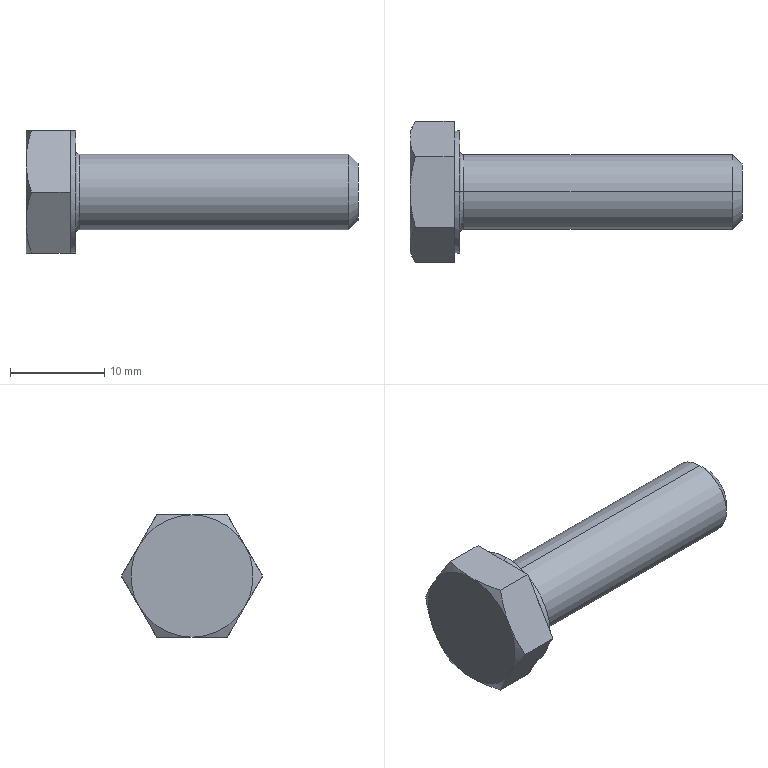Part | SolidWorks | features RevCut 4, Chamfer 1, Extrusion 1, Fillet 1, LPattern 1, Revolution 1 | 1 solid | 29 faces | box 35.3 x 15.011 x 13 mm | volume 2262 mm3 | plane 15 | cone 8 | cylinder 4 | torus 2 | commonest cylinder face diameters 8 x2 13 x2
STEP:
#1=CARTESIAN_POINT('',(5.7,0.,4.));
#2=VERTEX_POINT('',#1);
#3=CARTESIAN_POINT('',(5.7,0.,-4.));
#4=VERTEX_POINT('',#3);
#5=CARTESIAN_POINT('',(5.7,0.,0.));
#6=DIRECTION('',(1.,0.,0.));
#7=DIRECTION('',(0.,0.,-1.));
#8=AXIS2_PLACEMENT_3D('',#5,#6,#7);
#9=CIRCLE('',#8,4.);
#10=EDGE_CURVE('',#2,#4,#9,.T.);
#11=ORIENTED_EDGE('',*,*,#10,.F.);
#12=CARTESIAN_POINT('',(5.3,0.,4.4));
#13=VERTEX_POINT('',#12);
#14=CARTESIAN_POINT('',(5.7,0.,4.4));
#15=DIRECTION('',(0.,1.,0.));
#16=DIRECTION('',(0.,0.,1.));
#17=AXIS2_PLACEMENT_3D('',#14,#15,#16);
#18=CIRCLE('',#17,0.4);
#19=EDGE_CURVE('',#2,#13,#18,.T.);
#20=ORIENTED_EDGE('',*,*,#19,.T.);
#21=CARTESIAN_POINT('',(5.3,0.,-4.4));
#22=VERTEX_POINT('',#21);
#23=CARTESIAN_POINT('',(5.3,0.,0.));
#24=DIRECTION('',(-1.,0.,0.));
#25=DIRECTION('',(0.,0.,-1.));
#26=AXIS2_PLACEMENT_3D('',#23,#24,#25);
#27=CIRCLE('',#26,4.4);
#28=EDGE_CURVE('',#22,#13,#27,.T.);
#29=ORIENTED_EDGE('',*,*,#28,.F.);
#30=CARTESIAN_POINT('',(5.7,0.,-4.4));
#31=DIRECTION('',(0.,-1.,0.));
#32=DIRECTION('',(0.,0.,-1.));
#33=AXIS2_PLACEMENT_3D('',#30,#31,#32);
#34=CIRCLE('',#33,0.4);
#35=EDGE_CURVE('',#4,#22,#34,.T.);
#36=ORIENTED_EDGE('',*,*,#35,.F.);
#37=EDGE_LOOP('',(#11,#20,#29,#36));
#38=FACE_OUTER_BOUND('',#37,.T.);
#39=CARTESIAN_POINT('',(5.7,0.,0.));
#40=DIRECTION('',(1.,0.,0.));
#41=DIRECTION('',(0.,0.,-1.));
#42=AXIS2_PLACEMENT_3D('',#39,#40,#41);
#43=TOROIDAL_SURFACE('',#42,4.4,0.4);
#44=ADVANCED_FACE('',(#38),#43,.F.);
#45=CARTESIAN_POINT('',(35.3,0.,-3.));
#46=VERTEX_POINT('',#45);
#47=CARTESIAN_POINT('',(35.3,0.,3.));
#48=VERTEX_POINT('',#47);
#49=CARTESIAN_POINT('',(35.3,0.,0.));
#50=DIRECTION('',(1.,0.,0.));
#51=DIRECTION('',(0.,0.,1.));
#52=AXIS2_PLACEMENT_3D('',#49,#50,#51);
#53=CIRCLE('',#52,3.);
#54=EDGE_CURVE('',#46,#48,#53,.T.);
#55=ORIENTED_EDGE('',*,*,#54,.F.);
#56=CARTESIAN_POINT('',(34.3,0.,-4.));
#57=VERTEX_POINT('',#56);
#58=CARTESIAN_POINT('',(34.3,0.,-4.));
#59=DIRECTION('',(-0.7071,0.,-0.7071));
#60=VECTOR('',#59,1000.);
#61=LINE('',#58,#60);
#62=EDGE_CURVE('',#46,#57,#61,.T.);
#63=ORIENTED_EDGE('',*,*,#62,.T.);
#64=CARTESIAN_POINT('',(34.3,0.,4.));
#65=VERTEX_POINT('',#64);
#66=CARTESIAN_POINT('',(34.3,0.,0.));
#67=DIRECTION('',(-1.,0.,0.));
#68=DIRECTION('',(0.,0.,1.));
#69=AXIS2_PLACEMENT_3D('',#66,#67,#68);
#70=CIRCLE('',#69,4.);
#71=EDGE_CURVE('',#65,#57,#70,.T.);
#72=ORIENTED_EDGE('',*,*,#71,.F.);
#73=CARTESIAN_POINT('',(34.3,0.,4.));
#74=DIRECTION('',(-0.7071,0.,0.7071));
#75=VECTOR('',#74,1000.);
#76=LINE('',#73,#75);
#77=EDGE_CURVE('',#48,#65,#76,.T.);
#78=ORIENTED_EDGE('',*,*,#77,.F.);
#79=EDGE_LOOP('',(#55,#63,#72,#78));
#80=FACE_OUTER_BOUND('',#79,.T.);
#81=CARTESIAN_POINT('',(34.3,0.,0.));
#82=DIRECTION('',(-1.,0.,0.));
#83=DIRECTION('',(0.,0.,1.));
#84=AXIS2_PLACEMENT_3D('',#81,#82,#83);
#85=CONICAL_SURFACE('',#84,4.,0.7854);
#86=ADVANCED_FACE('',(#80),#85,.T.);
#87=ORIENTED_EDGE('',*,*,#71,.T.);
#88=CARTESIAN_POINT('',(0.,0.,-4.));
#89=DIRECTION('',(-1.,0.,0.));
#90=VECTOR('',#89,1000.);
#91=LINE('',#88,#90);
#92=EDGE_CURVE('',#57,#4,#91,.T.);
#93=ORIENTED_EDGE('',*,*,#92,.T.);
#94=CARTESIAN_POINT('',(5.7,0.,0.));
#95=DIRECTION('',(1.,0.,0.));
#96=DIRECTION('',(0.,0.,-1.));
#97=AXIS2_PLACEMENT_3D('',#94,#95,#96);
#98=CIRCLE('',#97,4.);
#99=EDGE_CURVE('',#4,#2,#98,.T.);
#100=ORIENTED_EDGE('',*,*,#99,.T.);
#101=CARTESIAN_POINT('',(0.,0.,4.));
#102=DIRECTION('',(-1.,0.,0.));
#103=VECTOR('',#102,1000.);
#104=LINE('',#101,#103);
#105=EDGE_CURVE('',#65,#2,#104,.T.);
#106=ORIENTED_EDGE('',*,*,#105,.F.);
#107=EDGE_LOOP('',(#87,#93,#100,#106));
#108=FACE_OUTER_BOUND('',#107,.T.);
#109=CARTESIAN_POINT('',(0.,0.,0.));
#110=DIRECTION('',(-1.,0.,0.));
#111=DIRECTION('',(0.,0.,1.));
#112=AXIS2_PLACEMENT_3D('',#109,#110,#111);
#113=CYLINDRICAL_SURFACE('',#112,4.);
#114=ADVANCED_FACE('',(#108),#113,.T.);
#115=CARTESIAN_POINT('',(5.3,0.,-6.5));
#116=VERTEX_POINT('',#115);
#117=CARTESIAN_POINT('',(5.3,0.,6.5));
#118=VERTEX_POINT('',#117);
#119=CARTESIAN_POINT('',(5.3,0.,0.));
#120=DIRECTION('',(1.,0.,0.));
#121=DIRECTION('',(0.,0.,-1.));
#122=AXIS2_PLACEMENT_3D('',#119,#120,#121);
#123=CIRCLE('',#122,6.5);
#124=EDGE_CURVE('',#116,#118,#123,.T.);
#125=ORIENTED_EDGE('',*,*,#124,.F.);
#126=CARTESIAN_POINT('',(4.7,0.,-6.5));
#127=VERTEX_POINT('',#126);
#128=CARTESIAN_POINT('',(0.,0.,-6.5));
#129=DIRECTION('',(-1.,0.,0.));
#130=VECTOR('',#129,1000.);
#131=LINE('',#128,#130);
#132=EDGE_CURVE('',#116,#127,#131,.T.);
#133=ORIENTED_EDGE('',*,*,#132,.T.);
#134=CARTESIAN_POINT('',(4.7,5.629,-3.25));
#135=VERTEX_POINT('',#134);
#136=CARTESIAN_POINT('',(4.7,0.,0.));
#137=DIRECTION('',(-1.,0.,0.));
#138=DIRECTION('',(0.,0.,1.));
#139=AXIS2_PLACEMENT_3D('',#136,#137,#138);
#140=CIRCLE('',#139,6.5);
#141=EDGE_CURVE('',#135,#127,#140,.T.);
#142=ORIENTED_EDGE('',*,*,#141,.F.);
#143=CARTESIAN_POINT('',(4.7,5.629,3.25));
#144=VERTEX_POINT('',#143);
#145=CARTESIAN_POINT('',(4.7,0.,0.));
#146=DIRECTION('',(-1.,0.,0.));
#147=DIRECTION('',(0.,0.,1.));
#148=AXIS2_PLACEMENT_3D('',#145,#146,#147);
#149=CIRCLE('',#148,6.5);
#150=EDGE_CURVE('',#144,#135,#149,.T.);
#151=ORIENTED_EDGE('',*,*,#150,.F.);
#152=CARTESIAN_POINT('',(4.7,0.,6.5));
#153=VERTEX_POINT('',#152);
#154=CARTESIAN_POINT('',(4.7,0.,0.));
#155=DIRECTION('',(-1.,0.,0.));
#156=DIRECTION('',(0.,0.,1.));
#157=AXIS2_PLACEMENT_3D('',#154,#155,#156);
#158=CIRCLE('',#157,6.5);
#159=EDGE_CURVE('',#153,#144,#158,.T.);
#160=ORIENTED_EDGE('',*,*,#159,.F.);
#161=CARTESIAN_POINT('',(0.,0.,6.5));
#162=DIRECTION('',(-1.,0.,0.));
#163=VECTOR('',#162,1000.);
#164=LINE('',#161,#163);
#165=EDGE_CURVE('',#118,#153,#164,.T.);
#166=ORIENTED_EDGE('',*,*,#165,.F.);
#167=EDGE_LOOP('',(#125,#133,#142,#151,#160,#166));
#168=FACE_OUTER_BOUND('',#167,.T.);
#169=CARTESIAN_POINT('',(0.,0.,0.));
#170=DIRECTION('',(-1.,0.,0.));
#171=DIRECTION('',(0.,0.,1.));
#172=AXIS2_PLACEMENT_3D('',#169,#170,#171);
#173=CYLINDRICAL_SURFACE('',#172,6.5);
#174=ADVANCED_FACE('',(#168),#173,.T.);
#175=CARTESIAN_POINT('',(4.7,3.753,-6.5));
#176=VERTEX_POINT('',#175);
#177=CARTESIAN_POINT('',(4.7,3.753,-6.5));
#178=DIRECTION('',(0.,0.5,0.866));
#179=VECTOR('',#178,1000.);
#180=LINE('',#177,#179);
#181=EDGE_CURVE('',#176,#135,#180,.T.);
#182=ORIENTED_EDGE('',*,*,#181,.F.);
#183=CARTESIAN_POINT('',(0.5806,3.753,-6.5));
#184=VERTEX_POINT('',#183);
#185=CARTESIAN_POINT('',(5.3,3.753,-6.5));
#186=DIRECTION('',(-1.,0.,0.));
#187=VECTOR('',#186,1000.);
#188=LINE('',#185,#187);
#189=EDGE_CURVE('',#176,#184,#188,.T.);
#190=ORIENTED_EDGE('',*,*,#189,.T.);
#191=CARTESIAN_POINT('',(0.,5.629,-3.25));
#192=VERTEX_POINT('',#191);
#193=CARTESIAN_POINT('',(0.,5.629,-3.25));
#194=CARTESIAN_POINT('',(0.,5.47,-3.526));
#195=CARTESIAN_POINT('',(0.01372,5.31,-3.803));
#196=CARTESIAN_POINT('',(0.06683,4.994,-4.351));
#197=CARTESIAN_POINT('',(0.1062,4.836,-4.623));
#198=CARTESIAN_POINT('',(0.2578,4.368,-5.435));
#199=CARTESIAN_POINT('',(0.4038,4.059,-5.97));
#200=CARTESIAN_POINT('',(0.5806,3.753,-6.5));
#201=B_SPLINE_CURVE_WITH_KNOTS('',3,(#193,#194,#195,#196,#197,#198,#199,#200),.UNSPECIFIED.,.F.,.F.,(4,2,2,4),(0.003797,0.004743,0.005689,0.00758),.UNSPECIFIED.);
#202=EDGE_CURVE('',#192,#184,#201,.T.);
#203=ORIENTED_EDGE('',*,*,#202,.F.);
#204=CARTESIAN_POINT('',(0.5806,7.506,0.));
#205=VERTEX_POINT('',#204);
#206=CARTESIAN_POINT('',(0.5806,7.506,0.));
#207=CARTESIAN_POINT('',(0.4033,7.199,-0.5317));
#208=CARTESIAN_POINT('',(0.2573,6.889,-1.067));
#209=CARTESIAN_POINT('',(0.05533,6.265,-2.149));
#210=CARTESIAN_POINT('',(0.,5.949,-2.696));
#211=CARTESIAN_POINT('',(0.,5.629,-3.25));
#212=B_SPLINE_CURVE_WITH_KNOTS('',3,(#206,#207,#208,#209,#210,#211),.UNSPECIFIED.,.F.,.F.,(4,2,4),(0.000000238,0.001899,0.003797),.UNSPECIFIED.);
#213=EDGE_CURVE('',#205,#192,#212,.T.);
#214=ORIENTED_EDGE('',*,*,#213,.F.);
#215=CARTESIAN_POINT('',(4.7,7.506,0.));
#216=VERTEX_POINT('',#215);
#217=CARTESIAN_POINT('',(5.3,7.506,0.));
#218=DIRECTION('',(-1.,0.,0.));
#219=VECTOR('',#218,1000.);
#220=LINE('',#217,#219);
#221=EDGE_CURVE('',#216,#205,#220,.T.);
#222=ORIENTED_EDGE('',*,*,#221,.F.);
#223=CARTESIAN_POINT('',(4.7,3.753,-6.5));
#224=DIRECTION('',(0.,0.5,0.866));
#225=VECTOR('',#224,1000.);
#226=LINE('',#223,#225);
#227=EDGE_CURVE('',#135,#216,#226,.T.);
#228=ORIENTED_EDGE('',*,*,#227,.F.);
#229=EDGE_LOOP('',(#182,#190,#203,#214,#222,#228));
#230=FACE_OUTER_BOUND('',#229,.T.);
#231=CARTESIAN_POINT('',(5.3,3.753,-6.5));
#232=DIRECTION('',(0.,-0.866,0.5));
#233=DIRECTION('',(0.,-0.5,-0.866));
#234=AXIS2_PLACEMENT_3D('',#231,#232,#233);
#235=PLANE('',#234);
#236=ADVANCED_FACE('',(#230),#235,.F.);
#237=CARTESIAN_POINT('',(4.7,7.506,0.));
#238=DIRECTION('',(0.,-0.5,0.866));
#239=VECTOR('',#238,1000.);
#240=LINE('',#237,#239);
#241=EDGE_CURVE('',#216,#144,#240,.T.);
#242=ORIENTED_EDGE('',*,*,#241,.F.);
#243=ORIENTED_EDGE('',*,*,#221,.T.);
#244=CARTESIAN_POINT('',(0.,5.629,3.25));
#245=VERTEX_POINT('',#244);
#246=CARTESIAN_POINT('',(0.,5.629,3.25));
#247=CARTESIAN_POINT('',(0.,5.788,2.974));
#248=CARTESIAN_POINT('',(0.01372,5.948,2.697));
#249=CARTESIAN_POINT('',(0.06683,6.265,2.149));
#250=CARTESIAN_POINT('',(0.1062,6.422,1.877));
#251=CARTESIAN_POINT('',(0.2578,6.891,1.065));
#252=CARTESIAN_POINT('',(0.4038,7.199,0.5303));
#253=CARTESIAN_POINT('',(0.5806,7.506,0.));
#254=B_SPLINE_CURVE_WITH_KNOTS('',3,(#246,#247,#248,#249,#250,#251,#252,#253),.UNSPECIFIED.,.F.,.F.,(4,2,2,4),(0.003797,0.004743,0.005689,0.00758),.UNSPECIFIED.);
#255=EDGE_CURVE('',#245,#205,#254,.T.);
#256=ORIENTED_EDGE('',*,*,#255,.F.);
#257=CARTESIAN_POINT('',(0.5806,3.753,6.5));
#258=VERTEX_POINT('',#257);
#259=CARTESIAN_POINT('',(0.5806,3.753,6.5));
#260=CARTESIAN_POINT('',(0.4033,4.06,5.968));
#261=CARTESIAN_POINT('',(0.2573,4.369,5.433));
#262=CARTESIAN_POINT('',(0.05533,4.994,4.351));
#263=CARTESIAN_POINT('',(0.,5.309,3.804));
#264=CARTESIAN_POINT('',(0.,5.629,3.25));
#265=B_SPLINE_CURVE_WITH_KNOTS('',3,(#259,#260,#261,#262,#263,#264),.UNSPECIFIED.,.F.,.F.,(4,2,4),(0.000000238,0.001899,0.003797),.UNSPECIFIED.);
#266=EDGE_CURVE('',#258,#245,#265,.T.);
#267=ORIENTED_EDGE('',*,*,#266,.F.);
#268=CARTESIAN_POINT('',(4.7,3.753,6.5));
#269=VERTEX_POINT('',#268);
#270=CARTESIAN_POINT('',(5.3,3.753,6.5));
#271=DIRECTION('',(-1.,0.,0.));
#272=VECTOR('',#271,1000.);
#273=LINE('',#270,#272);
#274=EDGE_CURVE('',#269,#258,#273,.T.);
#275=ORIENTED_EDGE('',*,*,#274,.F.);
#276=CARTESIAN_POINT('',(4.7,7.506,0.));
#277=DIRECTION('',(0.,-0.5,0.866));
#278=VECTOR('',#277,1000.);
#279=LINE('',#276,#278);
#280=EDGE_CURVE('',#144,#269,#279,.T.);
#281=ORIENTED_EDGE('',*,*,#280,.F.);
#282=EDGE_LOOP('',(#242,#243,#256,#267,#275,#281));
#283=FACE_OUTER_BOUND('',#282,.T.);
#284=CARTESIAN_POINT('',(5.3,7.506,0.));
#285=DIRECTION('',(0.,-0.866,-0.5));
#286=DIRECTION('',(0.,0.5,-0.866));
#287=AXIS2_PLACEMENT_3D('',#284,#285,#286);
#288=PLANE('',#287);
#289=ADVANCED_FACE('',(#283),#288,.F.);
#290=CARTESIAN_POINT('',(4.7,3.753,6.5));
#291=DIRECTION('',(0.,-1.,0.));
#292=VECTOR('',#291,1000.);
#293=LINE('',#290,#292);
#294=EDGE_CURVE('',#269,#153,#293,.T.);
#295=ORIENTED_EDGE('',*,*,#294,.F.);
#296=ORIENTED_EDGE('',*,*,#274,.T.);
#297=CARTESIAN_POINT('',(0.,0.,6.5));
#298=VERTEX_POINT('',#297);
#299=CARTESIAN_POINT('',(0.,0.,6.5));
#300=CARTESIAN_POINT('',(0.,0.6351,6.5));
#301=CARTESIAN_POINT('',(0.05613,1.279,6.5));
#302=CARTESIAN_POINT('',(0.2595,2.531,6.5));
#303=CARTESIAN_POINT('',(0.4054,3.146,6.5));
#304=CARTESIAN_POINT('',(0.5806,3.753,6.5));
#305=B_SPLINE_CURVE_WITH_KNOTS('',3,(#299,#300,#301,#302,#303,#304),.UNSPECIFIED.,.F.,.F.,(4,2,4),(0.01067,0.01257,0.01447),.UNSPECIFIED.);
#306=EDGE_CURVE('',#298,#258,#305,.T.);
#307=ORIENTED_EDGE('',*,*,#306,.F.);
#308=CARTESIAN_POINT('',(0.5806,-3.753,6.5));
#309=VERTEX_POINT('',#308);
#310=CARTESIAN_POINT('',(0.5806,-3.753,6.5));
#311=CARTESIAN_POINT('',(0.4042,-3.142,6.5));
#312=CARTESIAN_POINT('',(0.2565,-2.517,6.5));
#313=CARTESIAN_POINT('',(0.05459,-1.265,6.5));
#314=CARTESIAN_POINT('',(0.,-0.6347,6.5));
#315=CARTESIAN_POINT('',(0.,0.,6.5));
#316=B_SPLINE_CURVE_WITH_KNOTS('',3,(#310,#311,#312,#313,#314,#315),.UNSPECIFIED.,.F.,.F.,(4,2,4),(0.006874,0.008773,0.01067),.UNSPECIFIED.);
#317=EDGE_CURVE('',#309,#298,#316,.T.);
#318=ORIENTED_EDGE('',*,*,#317,.F.);
#319=CARTESIAN_POINT('',(4.7,-3.753,6.5));
#320=VERTEX_POINT('',#319);
#321=CARTESIAN_POINT('',(5.3,-3.753,6.5));
#322=DIRECTION('',(-1.,0.,0.));
#323=VECTOR('',#322,1000.);
#324=LINE('',#321,#323);
#325=EDGE_CURVE('',#320,#309,#324,.T.);
#326=ORIENTED_EDGE('',*,*,#325,.F.);
#327=CARTESIAN_POINT('',(4.7,3.753,6.5));
#328=DIRECTION('',(0.,-1.,0.));
#329=VECTOR('',#328,1000.);
#330=LINE('',#327,#329);
#331=EDGE_CURVE('',#153,#320,#330,.T.);
#332=ORIENTED_EDGE('',*,*,#331,.F.);
#333=EDGE_LOOP('',(#295,#296,#307,#318,#326,#332));
#334=FACE_OUTER_BOUND('',#333,.T.);
#335=CARTESIAN_POINT('',(5.3,3.753,6.5));
#336=DIRECTION('',(0.,0.,-1.));
#337=DIRECTION('',(-1.,0.,0.));
#338=AXIS2_PLACEMENT_3D('',#335,#336,#337);
#339=PLANE('',#338);
#340=ADVANCED_FACE('',(#334),#339,.F.);
#341=CARTESIAN_POINT('',(4.7,-5.629,3.25));
#342=VERTEX_POINT('',#341);
#343=CARTESIAN_POINT('',(4.7,-7.506,0.));
#344=DIRECTION('',(0.,-0.5,-0.866));
#345=VECTOR('',#344,1000.);
#346=LINE('',#343,#345);
#347=EDGE_CURVE('',#320,#342,#346,.T.);
#348=ORIENTED_EDGE('',*,*,#347,.F.);
#349=ORIENTED_EDGE('',*,*,#325,.T.);
#350=CARTESIAN_POINT('',(0.,-5.629,3.25));
#351=VERTEX_POINT('',#350);
#352=CARTESIAN_POINT('',(0.,-5.629,3.25));
#353=CARTESIAN_POINT('',(0.,-5.47,3.526));
#354=CARTESIAN_POINT('',(0.01372,-5.31,3.803));
#355=CARTESIAN_POINT('',(0.06683,-4.994,4.351));
#356=CARTESIAN_POINT('',(0.1062,-4.836,4.623));
#357=CARTESIAN_POINT('',(0.2578,-4.368,5.435));
#358=CARTESIAN_POINT('',(0.4038,-4.059,5.97));
#359=CARTESIAN_POINT('',(0.5806,-3.753,6.5));
#360=B_SPLINE_CURVE_WITH_KNOTS('',3,(#352,#353,#354,#355,#356,#357,#358,#359),.UNSPECIFIED.,.F.,.F.,(4,2,2,4),(0.003797,0.004743,0.005689,0.00758),.UNSPECIFIED.);
#361=EDGE_CURVE('',#351,#309,#360,.T.);
#362=ORIENTED_EDGE('',*,*,#361,.F.);
#363=CARTESIAN_POINT('',(0.5806,-7.506,0.));
#364=VERTEX_POINT('',#363);
#365=CARTESIAN_POINT('',(0.5806,-7.506,0.));
#366=CARTESIAN_POINT('',(0.4033,-7.199,0.5317));
#367=CARTESIAN_POINT('',(0.2573,-6.889,1.067));
#368=CARTESIAN_POINT('',(0.05533,-6.265,2.149));
#369=CARTESIAN_POINT('',(0.,-5.949,2.696));
#370=CARTESIAN_POINT('',(0.,-5.629,3.25));
#371=B_SPLINE_CURVE_WITH_KNOTS('',3,(#365,#366,#367,#368,#369,#370),.UNSPECIFIED.,.F.,.F.,(4,2,4),(0.000000238,0.001899,0.003797),.UNSPECIFIED.);
#372=EDGE_CURVE('',#364,#351,#371,.T.);
#373=ORIENTED_EDGE('',*,*,#372,.F.);
#374=CARTESIAN_POINT('',(4.7,-7.506,0.));
#375=VERTEX_POINT('',#374);
#376=CARTESIAN_POINT('',(5.3,-7.506,0.));
#377=DIRECTION('',(-1.,0.,0.));
#378=VECTOR('',#377,1000.);
#379=LINE('',#376,#378);
#380=EDGE_CURVE('',#375,#364,#379,.T.);
#381=ORIENTED_EDGE('',*,*,#380,.F.);
#382=CARTESIAN_POINT('',(4.7,-7.506,0.));
#383=DIRECTION('',(0.,-0.5,-0.866));
#384=VECTOR('',#383,1000.);
#385=LINE('',#382,#384);
#386=EDGE_CURVE('',#342,#375,#385,.T.);
#387=ORIENTED_EDGE('',*,*,#386,.F.);
#388=EDGE_LOOP('',(#348,#349,#362,#373,#381,#387));
#389=FACE_OUTER_BOUND('',#388,.T.);
#390=CARTESIAN_POINT('',(5.3,-7.506,0.));
#391=DIRECTION('',(0.,0.866,-0.5));
#392=DIRECTION('',(0.,0.5,0.866));
#393=AXIS2_PLACEMENT_3D('',#390,#391,#392);
#394=PLANE('',#393);
#395=ADVANCED_FACE('',(#389),#394,.F.);
#396=CARTESIAN_POINT('',(4.7,-5.629,-3.25));
#397=VERTEX_POINT('',#396);
#398=CARTESIAN_POINT('',(4.7,-3.753,-6.5));
#399=DIRECTION('',(0.,0.5,-0.866));
#400=VECTOR('',#399,1000.);
#401=LINE('',#398,#400);
#402=EDGE_CURVE('',#375,#397,#401,.T.);
#403=ORIENTED_EDGE('',*,*,#402,.F.);
#404=ORIENTED_EDGE('',*,*,#380,.T.);
#405=CARTESIAN_POINT('',(0.,-5.629,-3.25));
#406=VERTEX_POINT('',#405);
#407=CARTESIAN_POINT('',(0.,-5.629,-3.25));
#408=CARTESIAN_POINT('',(0.,-5.788,-2.974));
#409=CARTESIAN_POINT('',(0.01372,-5.948,-2.697));
#410=CARTESIAN_POINT('',(0.06683,-6.265,-2.149));
#411=CARTESIAN_POINT('',(0.1062,-6.422,-1.877));
#412=CARTESIAN_POINT('',(0.2578,-6.891,-1.065));
#413=CARTESIAN_POINT('',(0.4038,-7.199,-0.5303));
#414=CARTESIAN_POINT('',(0.5806,-7.506,0.));
#415=B_SPLINE_CURVE_WITH_KNOTS('',3,(#407,#408,#409,#410,#411,#412,#413,#414),.UNSPECIFIED.,.F.,.F.,(4,2,2,4),(0.003797,0.004743,0.005689,0.00758),.UNSPECIFIED.);
#416=EDGE_CURVE('',#406,#364,#415,.T.);
#417=ORIENTED_EDGE('',*,*,#416,.F.);
#418=CARTESIAN_POINT('',(0.5806,-3.753,-6.5));
#419=VERTEX_POINT('',#418);
#420=CARTESIAN_POINT('',(0.5806,-3.753,-6.5));
#421=CARTESIAN_POINT('',(0.4033,-4.06,-5.968));
#422=CARTESIAN_POINT('',(0.2573,-4.369,-5.433));
#423=CARTESIAN_POINT('',(0.05533,-4.994,-4.351));
#424=CARTESIAN_POINT('',(0.,-5.309,-3.804));
#425=CARTESIAN_POINT('',(0.,-5.629,-3.25));
#426=B_SPLINE_CURVE_WITH_KNOTS('',3,(#420,#421,#422,#423,#424,#425),.UNSPECIFIED.,.F.,.F.,(4,2,4),(0.000000238,0.001899,0.003797),.UNSPECIFIED.);
#427=EDGE_CURVE('',#419,#406,#426,.T.);
#428=ORIENTED_EDGE('',*,*,#427,.F.);
#429=CARTESIAN_POINT('',(4.7,-3.753,-6.5));
#430=VERTEX_POINT('',#429);
#431=CARTESIAN_POINT('',(5.3,-3.753,-6.5));
#432=DIRECTION('',(-1.,0.,0.));
#433=VECTOR('',#432,1000.);
#434=LINE('',#431,#433);
#435=EDGE_CURVE('',#430,#419,#434,.T.);
#436=ORIENTED_EDGE('',*,*,#435,.F.);
#437=CARTESIAN_POINT('',(4.7,-3.753,-6.5));
#438=DIRECTION('',(0.,0.5,-0.866));
#439=VECTOR('',#438,1000.);
#440=LINE('',#437,#439);
#441=EDGE_CURVE('',#397,#430,#440,.T.);
#442=ORIENTED_EDGE('',*,*,#441,.F.);
#443=EDGE_LOOP('',(#403,#404,#417,#428,#436,#442));
#444=FACE_OUTER_BOUND('',#443,.T.);
#445=CARTESIAN_POINT('',(5.3,-3.753,-6.5));
#446=DIRECTION('',(0.,0.866,0.5));
#447=DIRECTION('',(0.,-0.5,0.866));
#448=AXIS2_PLACEMENT_3D('',#445,#446,#447);
#449=PLANE('',#448);
#450=ADVANCED_FACE('',(#444),#449,.F.);
#451=CARTESIAN_POINT('',(4.7,3.753,-6.5));
#452=DIRECTION('',(0.,1.,0.));
#453=VECTOR('',#452,1000.);
#454=LINE('',#451,#453);
#455=EDGE_CURVE('',#430,#127,#454,.T.);
#456=ORIENTED_EDGE('',*,*,#455,.F.);
#457=ORIENTED_EDGE('',*,*,#435,.T.);
#458=CARTESIAN_POINT('',(0.,0.,-6.5));
#459=VERTEX_POINT('',#458);
#460=CARTESIAN_POINT('',(0.,0.,-6.5));
#461=CARTESIAN_POINT('',(0.,-0.6347,-6.5));
#462=CARTESIAN_POINT('',(0.05459,-1.265,-6.5));
#463=CARTESIAN_POINT('',(0.2565,-2.517,-6.5));
#464=CARTESIAN_POINT('',(0.4042,-3.142,-6.5));
#465=CARTESIAN_POINT('',(0.5806,-3.753,-6.5));
#466=B_SPLINE_CURVE_WITH_KNOTS('',3,(#460,#461,#462,#463,#464,#465),.UNSPECIFIED.,.F.,.F.,(4,2,4),(0.02294,0.02484,0.02674),.UNSPECIFIED.);
#467=EDGE_CURVE('',#459,#419,#466,.T.);
#468=ORIENTED_EDGE('',*,*,#467,.F.);
#469=CARTESIAN_POINT('',(0.5806,3.753,-6.5));
#470=CARTESIAN_POINT('',(0.4054,3.146,-6.5));
#471=CARTESIAN_POINT('',(0.2595,2.531,-6.5));
#472=CARTESIAN_POINT('',(0.05613,1.279,-6.5));
#473=CARTESIAN_POINT('',(0.,0.6351,-6.5));
#474=CARTESIAN_POINT('',(0.,0.,-6.5));
#475=B_SPLINE_CURVE_WITH_KNOTS('',3,(#469,#470,#471,#472,#473,#474),.UNSPECIFIED.,.F.,.F.,(4,2,4),(0.01914,0.02104,0.02294),.UNSPECIFIED.);
#476=EDGE_CURVE('',#184,#459,#475,.T.);
#477=ORIENTED_EDGE('',*,*,#476,.F.);
#478=ORIENTED_EDGE('',*,*,#189,.F.);
#479=CARTESIAN_POINT('',(4.7,3.753,-6.5));
#480=DIRECTION('',(0.,1.,0.));
#481=VECTOR('',#480,1000.);
#482=LINE('',#479,#481);
#483=EDGE_CURVE('',#127,#176,#482,.T.);
#484=ORIENTED_EDGE('',*,*,#483,.F.);
#485=EDGE_LOOP('',(#456,#457,#468,#477,#478,#484));
#486=FACE_OUTER_BOUND('',#485,.T.);
#487=CARTESIAN_POINT('',(5.3,3.753,-6.5));
#488=DIRECTION('',(0.,0.,1.));
#489=DIRECTION('',(0.,-1.,0.));
#490=AXIS2_PLACEMENT_3D('',#487,#488,#489);
#491=PLANE('',#490);
#492=ADVANCED_FACE('',(#486),#491,.F.);
#493=ORIENTED_EDGE('',*,*,#427,.T.);
#494=CARTESIAN_POINT('',(0.,0.,0.));
#495=DIRECTION('',(1.,0.,0.));
#496=DIRECTION('',(0.,0.,-1.));
#497=AXIS2_PLACEMENT_3D('',#494,#495,#496);
#498=CIRCLE('',#497,6.5);
#499=EDGE_CURVE('',#406,#459,#498,.T.);
#500=ORIENTED_EDGE('',*,*,#499,.T.);
#501=ORIENTED_EDGE('',*,*,#467,.T.);
#502=EDGE_LOOP('',(#493,#500,#501));
#503=FACE_OUTER_BOUND('',#502,.T.);
#504=CARTESIAN_POINT('',(0.,0.,0.));
#505=DIRECTION('',(1.,0.,0.));
#506=DIRECTION('',(0.,0.,-1.));
#507=AXIS2_PLACEMENT_3D('',#504,#505,#506);
#508=CONICAL_SURFACE('',#507,6.5,1.047);
#509=ADVANCED_FACE('',(#503),#508,.T.);
#510=ORIENTED_EDGE('',*,*,#372,.T.);
#511=CARTESIAN_POINT('',(0.,0.,0.));
#512=DIRECTION('',(1.,0.,0.));
#513=DIRECTION('',(0.,0.,-1.));
#514=AXIS2_PLACEMENT_3D('',#511,#512,#513);
#515=CIRCLE('',#514,6.5);
#516=EDGE_CURVE('',#351,#406,#515,.T.);
#517=ORIENTED_EDGE('',*,*,#516,.T.);
#518=ORIENTED_EDGE('',*,*,#416,.T.);
#519=EDGE_LOOP('',(#510,#517,#518));
#520=FACE_OUTER_BOUND('',#519,.T.);
#521=CARTESIAN_POINT('',(0.,0.,0.));
#522=DIRECTION('',(1.,0.,0.));
#523=DIRECTION('',(0.,0.,-1.));
#524=AXIS2_PLACEMENT_3D('',#521,#522,#523);
#525=CONICAL_SURFACE('',#524,6.5,1.047);
#526=ADVANCED_FACE('',(#520),#525,.T.);
#527=ORIENTED_EDGE('',*,*,#317,.T.);
#528=CARTESIAN_POINT('',(0.,0.,0.));
#529=DIRECTION('',(1.,0.,0.));
#530=DIRECTION('',(0.,0.,-1.));
#531=AXIS2_PLACEMENT_3D('',#528,#529,#530);
#532=CIRCLE('',#531,6.5);
#533=EDGE_CURVE('',#298,#351,#532,.T.);
#534=ORIENTED_EDGE('',*,*,#533,.T.);
#535=ORIENTED_EDGE('',*,*,#361,.T.);
#536=EDGE_LOOP('',(#527,#534,#535));
#537=FACE_OUTER_BOUND('',#536,.T.);
#538=CARTESIAN_POINT('',(0.,0.,0.));
#539=DIRECTION('',(1.,0.,0.));
#540=DIRECTION('',(0.,0.,-1.));
#541=AXIS2_PLACEMENT_3D('',#538,#539,#540);
#542=CONICAL_SURFACE('',#541,6.5,1.047);
#543=ADVANCED_FACE('',(#537),#542,.T.);
#544=ORIENTED_EDGE('',*,*,#306,.T.);
#545=ORIENTED_EDGE('',*,*,#266,.T.);
#546=CARTESIAN_POINT('',(0.,0.,0.));
#547=DIRECTION('',(-1.,0.,0.));
#548=DIRECTION('',(0.,0.,1.));
#549=AXIS2_PLACEMENT_3D('',#546,#547,#548);
#550=CIRCLE('',#549,6.5);
#551=EDGE_CURVE('',#298,#245,#550,.T.);
#552=ORIENTED_EDGE('',*,*,#551,.F.);
#553=EDGE_LOOP('',(#544,#545,#552));
#554=FACE_OUTER_BOUND('',#553,.T.);
#555=CARTESIAN_POINT('',(0.,0.,0.));
#556=DIRECTION('',(1.,0.,0.));
#557=DIRECTION('',(0.,0.,-1.));
#558=AXIS2_PLACEMENT_3D('',#555,#556,#557);
#559=CONICAL_SURFACE('',#558,6.5,1.047);
#560=ADVANCED_FACE('',(#554),#559,.T.);
#561=ORIENTED_EDGE('',*,*,#255,.T.);
#562=ORIENTED_EDGE('',*,*,#213,.T.);
#563=CARTESIAN_POINT('',(0.,0.,0.));
#564=DIRECTION('',(1.,0.,0.));
#565=DIRECTION('',(0.,0.,-1.));
#566=AXIS2_PLACEMENT_3D('',#563,#564,#565);
#567=CIRCLE('',#566,6.5);
#568=EDGE_CURVE('',#192,#245,#567,.T.);
#569=ORIENTED_EDGE('',*,*,#568,.T.);
#570=EDGE_LOOP('',(#561,#562,#569));
#571=FACE_OUTER_BOUND('',#570,.T.);
#572=CARTESIAN_POINT('',(0.,0.,0.));
#573=DIRECTION('',(1.,0.,0.));
#574=DIRECTION('',(0.,0.,-1.));
#575=AXIS2_PLACEMENT_3D('',#572,#573,#574);
#576=CONICAL_SURFACE('',#575,6.5,1.047);
#577=ADVANCED_FACE('',(#571),#576,.T.);
#578=ORIENTED_EDGE('',*,*,#202,.T.);
#579=ORIENTED_EDGE('',*,*,#476,.T.);
#580=CARTESIAN_POINT('',(0.,0.,0.));
#581=DIRECTION('',(1.,0.,0.));
#582=DIRECTION('',(0.,0.,-1.));
#583=AXIS2_PLACEMENT_3D('',#580,#581,#582);
#584=CIRCLE('',#583,6.5);
#585=EDGE_CURVE('',#459,#192,#584,.T.);
#586=ORIENTED_EDGE('',*,*,#585,.T.);
#587=EDGE_LOOP('',(#578,#579,#586));
#588=FACE_OUTER_BOUND('',#587,.T.);
#589=CARTESIAN_POINT('',(0.,0.,0.));
#590=DIRECTION('',(1.,0.,0.));
#591=DIRECTION('',(0.,0.,-1.));
#592=AXIS2_PLACEMENT_3D('',#589,#590,#591);
#593=CONICAL_SURFACE('',#592,6.5,1.047);
#594=ADVANCED_FACE('',(#588),#593,.T.);
#595=ORIENTED_EDGE('',*,*,#585,.F.);
#596=ORIENTED_EDGE('',*,*,#499,.F.);
#597=ORIENTED_EDGE('',*,*,#516,.F.);
#598=ORIENTED_EDGE('',*,*,#533,.F.);
#599=ORIENTED_EDGE('',*,*,#551,.T.);
#600=ORIENTED_EDGE('',*,*,#568,.F.);
#601=EDGE_LOOP('',(#595,#596,#597,#598,#599,#600));
#602=FACE_OUTER_BOUND('',#601,.T.);
#603=CARTESIAN_POINT('',(0.,7.506,0.));
#604=DIRECTION('',(1.,0.,0.));
#605=DIRECTION('',(0.,0.,-1.));
#606=AXIS2_PLACEMENT_3D('',#603,#604,#605);
#607=PLANE('',#606);
#608=ADVANCED_FACE('',(#602),#607,.F.);
#609=ORIENTED_EDGE('',*,*,#181,.T.);
#610=ORIENTED_EDGE('',*,*,#141,.T.);
#611=ORIENTED_EDGE('',*,*,#483,.T.);
#612=EDGE_LOOP('',(#609,#610,#611));
#613=FACE_OUTER_BOUND('',#612,.T.);
#614=CARTESIAN_POINT('',(4.7,6.5,0.));
#615=DIRECTION('',(1.,0.,0.));
#616=DIRECTION('',(0.,0.,-1.));
#617=AXIS2_PLACEMENT_3D('',#614,#615,#616);
#618=PLANE('',#617);
#619=ADVANCED_FACE('',(#613),#618,.T.);
#620=ORIENTED_EDGE('',*,*,#227,.T.);
#621=ORIENTED_EDGE('',*,*,#241,.T.);
#622=ORIENTED_EDGE('',*,*,#150,.T.);
#623=EDGE_LOOP('',(#620,#621,#622));
#624=FACE_OUTER_BOUND('',#623,.T.);
#625=CARTESIAN_POINT('',(4.7,6.5,0.));
#626=DIRECTION('',(1.,0.,0.));
#627=DIRECTION('',(0.,0.,-1.));
#628=AXIS2_PLACEMENT_3D('',#625,#626,#627);
#629=PLANE('',#628);
#630=ADVANCED_FACE('',(#624),#629,.T.);
#631=ORIENTED_EDGE('',*,*,#280,.T.);
#632=ORIENTED_EDGE('',*,*,#294,.T.);
#633=ORIENTED_EDGE('',*,*,#159,.T.);
#634=EDGE_LOOP('',(#631,#632,#633));
#635=FACE_OUTER_BOUND('',#634,.T.);
#636=CARTESIAN_POINT('',(4.7,6.5,0.));
#637=DIRECTION('',(1.,0.,0.));
#638=DIRECTION('',(0.,0.,-1.));
#639=AXIS2_PLACEMENT_3D('',#636,#637,#638);
#640=PLANE('',#639);
#641=ADVANCED_FACE('',(#635),#640,.T.);
#642=ORIENTED_EDGE('',*,*,#331,.T.);
#643=ORIENTED_EDGE('',*,*,#347,.T.);
#644=CARTESIAN_POINT('',(4.7,0.,0.));
#645=DIRECTION('',(-1.,0.,0.));
#646=DIRECTION('',(0.,0.,1.));
#647=AXIS2_PLACEMENT_3D('',#644,#645,#646);
#648=CIRCLE('',#647,6.5);
#649=EDGE_CURVE('',#342,#153,#648,.T.);
#650=ORIENTED_EDGE('',*,*,#649,.T.);
#651=EDGE_LOOP('',(#642,#643,#650));
#652=FACE_OUTER_BOUND('',#651,.T.);
#653=CARTESIAN_POINT('',(4.7,6.5,0.));
#654=DIRECTION('',(1.,0.,0.));
#655=DIRECTION('',(0.,0.,-1.));
#656=AXIS2_PLACEMENT_3D('',#653,#654,#655);
#657=PLANE('',#656);
#658=ADVANCED_FACE('',(#652),#657,.T.);
#659=ORIENTED_EDGE('',*,*,#386,.T.);
#660=ORIENTED_EDGE('',*,*,#402,.T.);
#661=CARTESIAN_POINT('',(4.7,0.,0.));
#662=DIRECTION('',(-1.,0.,0.));
#663=DIRECTION('',(0.,0.,1.));
#664=AXIS2_PLACEMENT_3D('',#661,#662,#663);
#665=CIRCLE('',#664,6.5);
#666=EDGE_CURVE('',#397,#342,#665,.T.);
#667=ORIENTED_EDGE('',*,*,#666,.T.);
#668=EDGE_LOOP('',(#659,#660,#667));
#669=FACE_OUTER_BOUND('',#668,.T.);
#670=CARTESIAN_POINT('',(4.7,6.5,0.));
#671=DIRECTION('',(1.,0.,0.));
#672=DIRECTION('',(0.,0.,-1.));
#673=AXIS2_PLACEMENT_3D('',#670,#671,#672);
#674=PLANE('',#673);
#675=ADVANCED_FACE('',(#669),#674,.T.);
#676=ORIENTED_EDGE('',*,*,#441,.T.);
#677=ORIENTED_EDGE('',*,*,#455,.T.);
#678=CARTESIAN_POINT('',(4.7,0.,0.));
#679=DIRECTION('',(-1.,0.,0.));
#680=DIRECTION('',(0.,0.,1.));
#681=AXIS2_PLACEMENT_3D('',#678,#679,#680);
#682=CIRCLE('',#681,6.5);
#683=EDGE_CURVE('',#127,#397,#682,.T.);
#684=ORIENTED_EDGE('',*,*,#683,.T.);
#685=EDGE_LOOP('',(#676,#677,#684));
#686=FACE_OUTER_BOUND('',#685,.T.);
#687=CARTESIAN_POINT('',(4.7,6.5,0.));
#688=DIRECTION('',(1.,0.,0.));
#689=DIRECTION('',(0.,0.,-1.));
#690=AXIS2_PLACEMENT_3D('',#687,#688,#689);
#691=PLANE('',#690);
#692=ADVANCED_FACE('',(#686),#691,.T.);
#693=ORIENTED_EDGE('',*,*,#132,.F.);
#694=CARTESIAN_POINT('',(5.3,0.,0.));
#695=DIRECTION('',(1.,0.,0.));
#696=DIRECTION('',(0.,0.,-1.));
#697=AXIS2_PLACEMENT_3D('',#694,#695,#696);
#698=CIRCLE('',#697,6.5);
#699=EDGE_CURVE('',#118,#116,#698,.T.);
#700=ORIENTED_EDGE('',*,*,#699,.F.);
#701=ORIENTED_EDGE('',*,*,#165,.T.);
#702=ORIENTED_EDGE('',*,*,#649,.F.);
#703=ORIENTED_EDGE('',*,*,#666,.F.);
#704=ORIENTED_EDGE('',*,*,#683,.F.);
#705=EDGE_LOOP('',(#693,#700,#701,#702,#703,#704));
#706=FACE_OUTER_BOUND('',#705,.T.);
#707=CARTESIAN_POINT('',(0.,0.,0.));
#708=DIRECTION('',(-1.,0.,0.));
#709=DIRECTION('',(0.,0.,1.));
#710=AXIS2_PLACEMENT_3D('',#707,#708,#709);
#711=CYLINDRICAL_SURFACE('',#710,6.5);
#712=ADVANCED_FACE('',(#706),#711,.T.);
#713=CARTESIAN_POINT('',(35.3,0.,0.));
#714=DIRECTION('',(1.,0.,0.));
#715=DIRECTION('',(0.,0.,1.));
#716=AXIS2_PLACEMENT_3D('',#713,#714,#715);
#717=CIRCLE('',#716,3.);
#718=EDGE_CURVE('',#48,#46,#717,.T.);
#719=ORIENTED_EDGE('',*,*,#718,.T.);
#720=ORIENTED_EDGE('',*,*,#54,.T.);
#721=EDGE_LOOP('',(#719,#720));
#722=FACE_OUTER_BOUND('',#721,.T.);
#723=CARTESIAN_POINT('',(35.3,0.,0.));
#724=DIRECTION('',(-1.,0.,0.));
#725=DIRECTION('',(0.,0.,1.));
#726=AXIS2_PLACEMENT_3D('',#723,#724,#725);
#727=PLANE('',#726);
#728=ADVANCED_FACE('',(#722),#727,.F.);
#729=ORIENTED_EDGE('',*,*,#92,.F.);
#730=CARTESIAN_POINT('',(34.3,0.,0.));
#731=DIRECTION('',(-1.,0.,0.));
#732=DIRECTION('',(0.,0.,1.));
#733=AXIS2_PLACEMENT_3D('',#730,#731,#732);
#734=CIRCLE('',#733,4.);
#735=EDGE_CURVE('',#57,#65,#734,.T.);
#736=ORIENTED_EDGE('',*,*,#735,.T.);
#737=ORIENTED_EDGE('',*,*,#105,.T.);
#738=ORIENTED_EDGE('',*,*,#10,.T.);
#739=EDGE_LOOP('',(#729,#736,#737,#738));
#740=FACE_OUTER_BOUND('',#739,.T.);
#741=CARTESIAN_POINT('',(0.,0.,0.));
#742=DIRECTION('',(-1.,0.,0.));
#743=DIRECTION('',(0.,0.,1.));
#744=AXIS2_PLACEMENT_3D('',#741,#742,#743);
#745=CYLINDRICAL_SURFACE('',#744,4.);
#746=ADVANCED_FACE('',(#740),#745,.T.);
#747=ORIENTED_EDGE('',*,*,#28,.T.);
#748=CARTESIAN_POINT('',(5.3,0.,0.));
#749=DIRECTION('',(-1.,0.,0.));
#750=DIRECTION('',(0.,0.,-1.));
#751=AXIS2_PLACEMENT_3D('',#748,#749,#750);
#752=CIRCLE('',#751,4.4);
#753=EDGE_CURVE('',#13,#22,#752,.T.);
#754=ORIENTED_EDGE('',*,*,#753,.T.);
#755=EDGE_LOOP('',(#747,#754));
#756=FACE_BOUND('',#755,.T.);
#757=ORIENTED_EDGE('',*,*,#699,.T.);
#758=ORIENTED_EDGE('',*,*,#124,.T.);
#759=EDGE_LOOP('',(#757,#758));
#760=FACE_OUTER_BOUND('',#759,.T.);
#761=CARTESIAN_POINT('',(5.3,7.506,0.));
#762=DIRECTION('',(1.,0.,0.));
#763=DIRECTION('',(0.,0.,-1.));
#764=AXIS2_PLACEMENT_3D('',#761,#762,#763);
#765=PLANE('',#764);
#766=ADVANCED_FACE('',(#756,#760),#765,.T.);
#767=ORIENTED_EDGE('',*,*,#62,.F.);
#768=ORIENTED_EDGE('',*,*,#718,.F.);
#769=ORIENTED_EDGE('',*,*,#77,.T.);
#770=ORIENTED_EDGE('',*,*,#735,.F.);
#771=EDGE_LOOP('',(#767,#768,#769,#770));
#772=FACE_OUTER_BOUND('',#771,.T.);
#773=CARTESIAN_POINT('',(34.3,0.,0.));
#774=DIRECTION('',(-1.,0.,0.));
#775=DIRECTION('',(0.,0.,1.));
#776=AXIS2_PLACEMENT_3D('',#773,#774,#775);
#777=CONICAL_SURFACE('',#776,4.,0.7854);
#778=ADVANCED_FACE('',(#772),#777,.T.);
#779=ORIENTED_EDGE('',*,*,#19,.F.);
#780=ORIENTED_EDGE('',*,*,#99,.F.);
#781=ORIENTED_EDGE('',*,*,#35,.T.);
#782=ORIENTED_EDGE('',*,*,#753,.F.);
#783=EDGE_LOOP('',(#779,#780,#781,#782));
#784=FACE_OUTER_BOUND('',#783,.T.);
#785=CARTESIAN_POINT('',(5.7,0.,0.));
#786=DIRECTION('',(1.,0.,0.));
#787=DIRECTION('',(0.,0.,-1.));
#788=AXIS2_PLACEMENT_3D('',#785,#786,#787);
#789=TOROIDAL_SURFACE('',#788,4.4,0.4);
#790=ADVANCED_FACE('',(#784),#789,.F.);
#791=CLOSED_SHELL('',(#44,#86,#114,#174,#236,#289,#340,#395,#450,#492,#509,#526,#543,#560,#577,#594,#608,#619,#630,#641,#658,#675,#692,#712,#728,#746,#766,#778,#790));
#792=MANIFOLD_SOLID_BREP('',#791);
#793=CARTESIAN_POINT('',(0.,0.,0.));
#794=DIRECTION('',(0.,0.,1.));
#795=DIRECTION('',(1.,0.,0.));
#796=AXIS2_PLACEMENT_3D('',#793,#794,#795);
#797=(LENGTH_UNIT()NAMED_UNIT(*)SI_UNIT(.MILLI.,.METRE.));
#798=UNCERTAINTY_MEASURE_WITH_UNIT(LENGTH_MEASURE(0.00001),#797,'','');
#799=(NAMED_UNIT(*)PLANE_ANGLE_UNIT()SI_UNIT($,.RADIAN.));
#800=(NAMED_UNIT(*)SI_UNIT($,.STERADIAN.)SOLID_ANGLE_UNIT());
#801=(GEOMETRIC_REPRESENTATION_CONTEXT(3)GLOBAL_UNCERTAINTY_ASSIGNED_CONTEXT((#798))GLOBAL_UNIT_ASSIGNED_CONTEXT((#797,#799,#800))REPRESENTATION_CONTEXT('',''));
#802=ADVANCED_BREP_SHAPE_REPRESENTATION('',(#792,#796),#801);